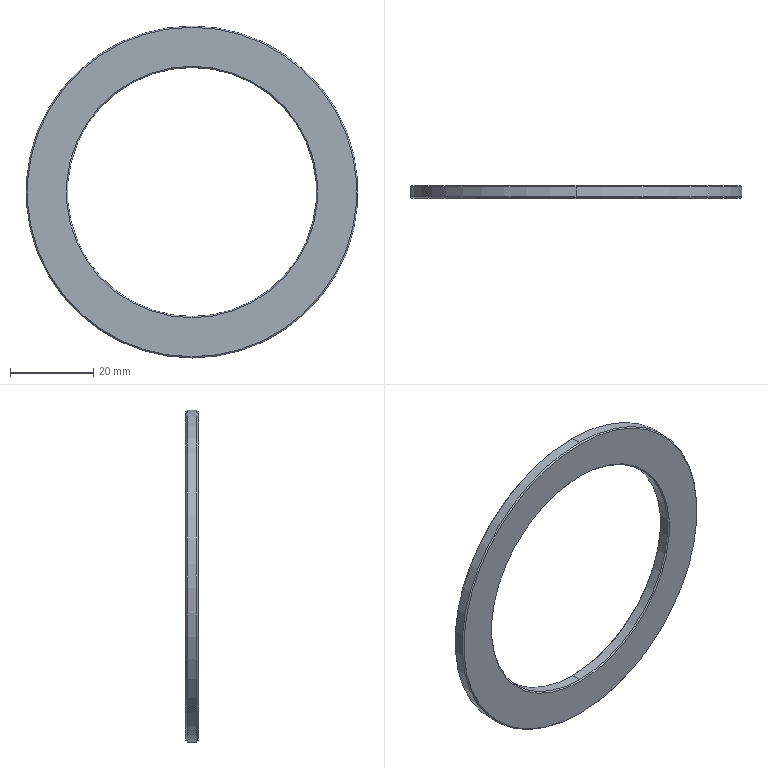Part | SolidWorks | features Chamfer 1, Extrusion 1 | 1 solid | 14 faces | box 80 x 3 x 80 mm | volume 6558 mm3 | cone 8 | cylinder 4 | plane 2 | commonest cylinder face diameters 60 x2 80 x2
STEP:
#1=CARTESIAN_POINT('',(0.,1.2,-30.));
#2=VERTEX_POINT('',#1);
#3=CARTESIAN_POINT('',(0.,1.2,30.));
#4=VERTEX_POINT('',#3);
#5=CARTESIAN_POINT('',(0.,1.2,0.));
#6=DIRECTION('',(0.,1.,0.));
#7=DIRECTION('',(0.,0.,1.));
#8=AXIS2_PLACEMENT_3D('',#5,#6,#7);
#9=CIRCLE('',#8,30.);
#10=EDGE_CURVE('',#2,#4,#9,.T.);
#11=ORIENTED_EDGE('',*,*,#10,.F.);
#12=CARTESIAN_POINT('',(0.,1.5,-30.3));
#13=VERTEX_POINT('',#12);
#14=CARTESIAN_POINT('',(0.,1.2,-30.));
#15=DIRECTION('',(0.,0.7071,-0.7071));
#16=VECTOR('',#15,1000.);
#17=LINE('',#14,#16);
#18=EDGE_CURVE('',#2,#13,#17,.T.);
#19=ORIENTED_EDGE('',*,*,#18,.T.);
#20=CARTESIAN_POINT('',(0.,1.5,30.3));
#21=VERTEX_POINT('',#20);
#22=CARTESIAN_POINT('',(0.,1.5,0.));
#23=DIRECTION('',(0.,-1.,0.));
#24=DIRECTION('',(0.,0.,1.));
#25=AXIS2_PLACEMENT_3D('',#22,#23,#24);
#26=CIRCLE('',#25,30.3);
#27=EDGE_CURVE('',#21,#13,#26,.T.);
#28=ORIENTED_EDGE('',*,*,#27,.F.);
#29=CARTESIAN_POINT('',(0.,1.2,30.));
#30=DIRECTION('',(0.,0.7071,0.7071));
#31=VECTOR('',#30,1000.);
#32=LINE('',#29,#31);
#33=EDGE_CURVE('',#4,#21,#32,.T.);
#34=ORIENTED_EDGE('',*,*,#33,.F.);
#35=EDGE_LOOP('',(#11,#19,#28,#34));
#36=FACE_OUTER_BOUND('',#35,.T.);
#37=CARTESIAN_POINT('',(0.,1.2,0.));
#38=DIRECTION('',(0.,1.,0.));
#39=DIRECTION('',(0.,0.,1.));
#40=AXIS2_PLACEMENT_3D('',#37,#38,#39);
#41=CONICAL_SURFACE('',#40,30.,0.7854);
#42=ADVANCED_FACE('',(#36),#41,.F.);
#43=CARTESIAN_POINT('',(0.,-1.2,30.));
#44=VERTEX_POINT('',#43);
#45=CARTESIAN_POINT('',(0.,-1.2,-30.));
#46=VERTEX_POINT('',#45);
#47=CARTESIAN_POINT('',(0.,-1.2,0.));
#48=DIRECTION('',(0.,-1.,0.));
#49=DIRECTION('',(0.,0.,1.));
#50=AXIS2_PLACEMENT_3D('',#47,#48,#49);
#51=CIRCLE('',#50,30.);
#52=EDGE_CURVE('',#44,#46,#51,.T.);
#53=ORIENTED_EDGE('',*,*,#52,.F.);
#54=CARTESIAN_POINT('',(0.,-1.5,30.3));
#55=VERTEX_POINT('',#54);
#56=CARTESIAN_POINT('',(0.,-1.5,30.3));
#57=DIRECTION('',(0.,-0.7071,0.7071));
#58=VECTOR('',#57,1000.);
#59=LINE('',#56,#58);
#60=EDGE_CURVE('',#44,#55,#59,.T.);
#61=ORIENTED_EDGE('',*,*,#60,.T.);
#62=CARTESIAN_POINT('',(0.,-1.5,-30.3));
#63=VERTEX_POINT('',#62);
#64=CARTESIAN_POINT('',(0.,-1.5,0.));
#65=DIRECTION('',(0.,1.,0.));
#66=DIRECTION('',(0.,0.,1.));
#67=AXIS2_PLACEMENT_3D('',#64,#65,#66);
#68=CIRCLE('',#67,30.3);
#69=EDGE_CURVE('',#63,#55,#68,.T.);
#70=ORIENTED_EDGE('',*,*,#69,.F.);
#71=CARTESIAN_POINT('',(0.,-1.5,-30.3));
#72=DIRECTION('',(0.,-0.7071,-0.7071));
#73=VECTOR('',#72,1000.);
#74=LINE('',#71,#73);
#75=EDGE_CURVE('',#46,#63,#74,.T.);
#76=ORIENTED_EDGE('',*,*,#75,.F.);
#77=EDGE_LOOP('',(#53,#61,#70,#76));
#78=FACE_OUTER_BOUND('',#77,.T.);
#79=CARTESIAN_POINT('',(0.,-1.5,0.));
#80=DIRECTION('',(0.,-1.,0.));
#81=DIRECTION('',(0.,0.,-1.));
#82=AXIS2_PLACEMENT_3D('',#79,#80,#81);
#83=CONICAL_SURFACE('',#82,30.3,0.7854);
#84=ADVANCED_FACE('',(#78),#83,.F.);
#85=CARTESIAN_POINT('',(0.,1.5,39.7));
#86=VERTEX_POINT('',#85);
#87=CARTESIAN_POINT('',(0.,1.5,-39.7));
#88=VERTEX_POINT('',#87);
#89=CARTESIAN_POINT('',(0.,1.5,0.));
#90=DIRECTION('',(0.,1.,0.));
#91=DIRECTION('',(0.,0.,1.));
#92=AXIS2_PLACEMENT_3D('',#89,#90,#91);
#93=CIRCLE('',#92,39.7);
#94=EDGE_CURVE('',#86,#88,#93,.T.);
#95=ORIENTED_EDGE('',*,*,#94,.F.);
#96=CARTESIAN_POINT('',(0.,1.2,40.));
#97=VERTEX_POINT('',#96);
#98=CARTESIAN_POINT('',(0.,1.5,39.7));
#99=DIRECTION('',(0.,-0.7071,0.7071));
#100=VECTOR('',#99,1000.);
#101=LINE('',#98,#100);
#102=EDGE_CURVE('',#86,#97,#101,.T.);
#103=ORIENTED_EDGE('',*,*,#102,.T.);
#104=CARTESIAN_POINT('',(0.,1.2,-40.));
#105=VERTEX_POINT('',#104);
#106=CARTESIAN_POINT('',(0.,1.2,0.));
#107=DIRECTION('',(0.,-1.,0.));
#108=DIRECTION('',(0.,0.,1.));
#109=AXIS2_PLACEMENT_3D('',#106,#107,#108);
#110=CIRCLE('',#109,40.);
#111=EDGE_CURVE('',#105,#97,#110,.T.);
#112=ORIENTED_EDGE('',*,*,#111,.F.);
#113=CARTESIAN_POINT('',(0.,1.5,-39.7));
#114=DIRECTION('',(0.,-0.7071,-0.7071));
#115=VECTOR('',#114,1000.);
#116=LINE('',#113,#115);
#117=EDGE_CURVE('',#88,#105,#116,.T.);
#118=ORIENTED_EDGE('',*,*,#117,.F.);
#119=EDGE_LOOP('',(#95,#103,#112,#118));
#120=FACE_OUTER_BOUND('',#119,.T.);
#121=CARTESIAN_POINT('',(0.,1.5,0.));
#122=DIRECTION('',(0.,-1.,0.));
#123=DIRECTION('',(0.,0.,-1.));
#124=AXIS2_PLACEMENT_3D('',#121,#122,#123);
#125=CONICAL_SURFACE('',#124,39.7,0.7854);
#126=ADVANCED_FACE('',(#120),#125,.T.);
#127=CARTESIAN_POINT('',(0.,-1.5,-39.7));
#128=VERTEX_POINT('',#127);
#129=CARTESIAN_POINT('',(0.,-1.5,39.7));
#130=VERTEX_POINT('',#129);
#131=CARTESIAN_POINT('',(0.,-1.5,0.));
#132=DIRECTION('',(0.,-1.,0.));
#133=DIRECTION('',(0.,0.,1.));
#134=AXIS2_PLACEMENT_3D('',#131,#132,#133);
#135=CIRCLE('',#134,39.7);
#136=EDGE_CURVE('',#128,#130,#135,.T.);
#137=ORIENTED_EDGE('',*,*,#136,.F.);
#138=CARTESIAN_POINT('',(0.,-1.2,-40.));
#139=VERTEX_POINT('',#138);
#140=CARTESIAN_POINT('',(0.,-1.2,-40.));
#141=DIRECTION('',(0.,0.7071,-0.7071));
#142=VECTOR('',#141,1000.);
#143=LINE('',#140,#142);
#144=EDGE_CURVE('',#128,#139,#143,.T.);
#145=ORIENTED_EDGE('',*,*,#144,.T.);
#146=CARTESIAN_POINT('',(0.,-1.2,40.));
#147=VERTEX_POINT('',#146);
#148=CARTESIAN_POINT('',(0.,-1.2,0.));
#149=DIRECTION('',(0.,1.,0.));
#150=DIRECTION('',(0.,0.,1.));
#151=AXIS2_PLACEMENT_3D('',#148,#149,#150);
#152=CIRCLE('',#151,40.);
#153=EDGE_CURVE('',#147,#139,#152,.T.);
#154=ORIENTED_EDGE('',*,*,#153,.F.);
#155=CARTESIAN_POINT('',(0.,-1.2,40.));
#156=DIRECTION('',(0.,0.7071,0.7071));
#157=VECTOR('',#156,1000.);
#158=LINE('',#155,#157);
#159=EDGE_CURVE('',#130,#147,#158,.T.);
#160=ORIENTED_EDGE('',*,*,#159,.F.);
#161=EDGE_LOOP('',(#137,#145,#154,#160));
#162=FACE_OUTER_BOUND('',#161,.T.);
#163=CARTESIAN_POINT('',(0.,-1.2,0.));
#164=DIRECTION('',(0.,1.,0.));
#165=DIRECTION('',(0.,0.,1.));
#166=AXIS2_PLACEMENT_3D('',#163,#164,#165);
#167=CONICAL_SURFACE('',#166,40.,0.7854);
#168=ADVANCED_FACE('',(#162),#167,.T.);
#169=ORIENTED_EDGE('',*,*,#10,.T.);
#170=CARTESIAN_POINT('',(0.,1.5,30.));
#171=DIRECTION('',(0.,-1.,0.));
#172=VECTOR('',#171,1000.);
#173=LINE('',#170,#172);
#174=EDGE_CURVE('',#4,#44,#173,.T.);
#175=ORIENTED_EDGE('',*,*,#174,.T.);
#176=ORIENTED_EDGE('',*,*,#52,.T.);
#177=CARTESIAN_POINT('',(0.,1.5,-30.));
#178=DIRECTION('',(0.,-1.,0.));
#179=VECTOR('',#178,1000.);
#180=LINE('',#177,#179);
#181=EDGE_CURVE('',#2,#46,#180,.T.);
#182=ORIENTED_EDGE('',*,*,#181,.F.);
#183=EDGE_LOOP('',(#169,#175,#176,#182));
#184=FACE_OUTER_BOUND('',#183,.T.);
#185=CARTESIAN_POINT('',(0.,1.5,0.));
#186=DIRECTION('',(0.,-1.,0.));
#187=DIRECTION('',(0.,0.,-1.));
#188=AXIS2_PLACEMENT_3D('',#185,#186,#187);
#189=CYLINDRICAL_SURFACE('',#188,30.);
#190=ADVANCED_FACE('',(#184),#189,.F.);
#191=ORIENTED_EDGE('',*,*,#111,.T.);
#192=CARTESIAN_POINT('',(0.,1.5,40.));
#193=DIRECTION('',(0.,-1.,0.));
#194=VECTOR('',#193,1000.);
#195=LINE('',#192,#194);
#196=EDGE_CURVE('',#97,#147,#195,.T.);
#197=ORIENTED_EDGE('',*,*,#196,.T.);
#198=ORIENTED_EDGE('',*,*,#153,.T.);
#199=CARTESIAN_POINT('',(0.,1.5,-40.));
#200=DIRECTION('',(0.,-1.,0.));
#201=VECTOR('',#200,1000.);
#202=LINE('',#199,#201);
#203=EDGE_CURVE('',#105,#139,#202,.T.);
#204=ORIENTED_EDGE('',*,*,#203,.F.);
#205=EDGE_LOOP('',(#191,#197,#198,#204));
#206=FACE_OUTER_BOUND('',#205,.T.);
#207=CARTESIAN_POINT('',(0.,1.5,0.));
#208=DIRECTION('',(0.,-1.,0.));
#209=DIRECTION('',(0.,0.,-1.));
#210=AXIS2_PLACEMENT_3D('',#207,#208,#209);
#211=CYLINDRICAL_SURFACE('',#210,40.);
#212=ADVANCED_FACE('',(#206),#211,.T.);
#213=CARTESIAN_POINT('',(0.,1.5,0.));
#214=DIRECTION('',(0.,1.,0.));
#215=DIRECTION('',(0.,0.,1.));
#216=AXIS2_PLACEMENT_3D('',#213,#214,#215);
#217=CIRCLE('',#216,39.7);
#218=EDGE_CURVE('',#88,#86,#217,.T.);
#219=ORIENTED_EDGE('',*,*,#218,.T.);
#220=ORIENTED_EDGE('',*,*,#94,.T.);
#221=EDGE_LOOP('',(#219,#220));
#222=FACE_OUTER_BOUND('',#221,.T.);
#223=ORIENTED_EDGE('',*,*,#27,.T.);
#224=CARTESIAN_POINT('',(0.,1.5,0.));
#225=DIRECTION('',(0.,-1.,0.));
#226=DIRECTION('',(0.,0.,1.));
#227=AXIS2_PLACEMENT_3D('',#224,#225,#226);
#228=CIRCLE('',#227,30.3);
#229=EDGE_CURVE('',#13,#21,#228,.T.);
#230=ORIENTED_EDGE('',*,*,#229,.T.);
#231=EDGE_LOOP('',(#223,#230));
#232=FACE_BOUND('',#231,.T.);
#233=CARTESIAN_POINT('',(0.,1.5,0.));
#234=DIRECTION('',(0.,1.,0.));
#235=DIRECTION('',(0.,0.,1.));
#236=AXIS2_PLACEMENT_3D('',#233,#234,#235);
#237=PLANE('',#236);
#238=ADVANCED_FACE('',(#222,#232),#237,.T.);
#239=CARTESIAN_POINT('',(0.,-1.5,0.));
#240=DIRECTION('',(0.,-1.,0.));
#241=DIRECTION('',(0.,0.,1.));
#242=AXIS2_PLACEMENT_3D('',#239,#240,#241);
#243=CIRCLE('',#242,39.7);
#244=EDGE_CURVE('',#130,#128,#243,.T.);
#245=ORIENTED_EDGE('',*,*,#244,.T.);
#246=ORIENTED_EDGE('',*,*,#136,.T.);
#247=EDGE_LOOP('',(#245,#246));
#248=FACE_OUTER_BOUND('',#247,.T.);
#249=ORIENTED_EDGE('',*,*,#69,.T.);
#250=CARTESIAN_POINT('',(0.,-1.5,0.));
#251=DIRECTION('',(0.,1.,0.));
#252=DIRECTION('',(0.,0.,1.));
#253=AXIS2_PLACEMENT_3D('',#250,#251,#252);
#254=CIRCLE('',#253,30.3);
#255=EDGE_CURVE('',#55,#63,#254,.T.);
#256=ORIENTED_EDGE('',*,*,#255,.T.);
#257=EDGE_LOOP('',(#249,#256));
#258=FACE_BOUND('',#257,.T.);
#259=CARTESIAN_POINT('',(0.,-1.5,0.));
#260=DIRECTION('',(0.,1.,0.));
#261=DIRECTION('',(0.,0.,1.));
#262=AXIS2_PLACEMENT_3D('',#259,#260,#261);
#263=PLANE('',#262);
#264=ADVANCED_FACE('',(#248,#258),#263,.F.);
#265=ORIENTED_EDGE('',*,*,#196,.F.);
#266=CARTESIAN_POINT('',(0.,1.2,0.));
#267=DIRECTION('',(0.,-1.,0.));
#268=DIRECTION('',(0.,0.,1.));
#269=AXIS2_PLACEMENT_3D('',#266,#267,#268);
#270=CIRCLE('',#269,40.);
#271=EDGE_CURVE('',#97,#105,#270,.T.);
#272=ORIENTED_EDGE('',*,*,#271,.T.);
#273=ORIENTED_EDGE('',*,*,#203,.T.);
#274=CARTESIAN_POINT('',(0.,-1.2,0.));
#275=DIRECTION('',(0.,1.,0.));
#276=DIRECTION('',(0.,0.,1.));
#277=AXIS2_PLACEMENT_3D('',#274,#275,#276);
#278=CIRCLE('',#277,40.);
#279=EDGE_CURVE('',#139,#147,#278,.T.);
#280=ORIENTED_EDGE('',*,*,#279,.T.);
#281=EDGE_LOOP('',(#265,#272,#273,#280));
#282=FACE_OUTER_BOUND('',#281,.T.);
#283=CARTESIAN_POINT('',(0.,1.5,0.));
#284=DIRECTION('',(0.,-1.,0.));
#285=DIRECTION('',(0.,0.,-1.));
#286=AXIS2_PLACEMENT_3D('',#283,#284,#285);
#287=CYLINDRICAL_SURFACE('',#286,40.);
#288=ADVANCED_FACE('',(#282),#287,.T.);
#289=ORIENTED_EDGE('',*,*,#174,.F.);
#290=CARTESIAN_POINT('',(0.,1.2,0.));
#291=DIRECTION('',(0.,1.,0.));
#292=DIRECTION('',(0.,0.,1.));
#293=AXIS2_PLACEMENT_3D('',#290,#291,#292);
#294=CIRCLE('',#293,30.);
#295=EDGE_CURVE('',#4,#2,#294,.T.);
#296=ORIENTED_EDGE('',*,*,#295,.T.);
#297=ORIENTED_EDGE('',*,*,#181,.T.);
#298=CARTESIAN_POINT('',(0.,-1.2,0.));
#299=DIRECTION('',(0.,-1.,0.));
#300=DIRECTION('',(0.,0.,1.));
#301=AXIS2_PLACEMENT_3D('',#298,#299,#300);
#302=CIRCLE('',#301,30.);
#303=EDGE_CURVE('',#46,#44,#302,.T.);
#304=ORIENTED_EDGE('',*,*,#303,.T.);
#305=EDGE_LOOP('',(#289,#296,#297,#304));
#306=FACE_OUTER_BOUND('',#305,.T.);
#307=CARTESIAN_POINT('',(0.,1.5,0.));
#308=DIRECTION('',(0.,-1.,0.));
#309=DIRECTION('',(0.,0.,-1.));
#310=AXIS2_PLACEMENT_3D('',#307,#308,#309);
#311=CYLINDRICAL_SURFACE('',#310,30.);
#312=ADVANCED_FACE('',(#306),#311,.F.);
#313=ORIENTED_EDGE('',*,*,#144,.F.);
#314=ORIENTED_EDGE('',*,*,#244,.F.);
#315=ORIENTED_EDGE('',*,*,#159,.T.);
#316=ORIENTED_EDGE('',*,*,#279,.F.);
#317=EDGE_LOOP('',(#313,#314,#315,#316));
#318=FACE_OUTER_BOUND('',#317,.T.);
#319=CARTESIAN_POINT('',(0.,-1.2,0.));
#320=DIRECTION('',(0.,1.,0.));
#321=DIRECTION('',(0.,0.,1.));
#322=AXIS2_PLACEMENT_3D('',#319,#320,#321);
#323=CONICAL_SURFACE('',#322,40.,0.7854);
#324=ADVANCED_FACE('',(#318),#323,.T.);
#325=ORIENTED_EDGE('',*,*,#102,.F.);
#326=ORIENTED_EDGE('',*,*,#218,.F.);
#327=ORIENTED_EDGE('',*,*,#117,.T.);
#328=ORIENTED_EDGE('',*,*,#271,.F.);
#329=EDGE_LOOP('',(#325,#326,#327,#328));
#330=FACE_OUTER_BOUND('',#329,.T.);
#331=CARTESIAN_POINT('',(0.,1.5,0.));
#332=DIRECTION('',(0.,-1.,0.));
#333=DIRECTION('',(0.,0.,-1.));
#334=AXIS2_PLACEMENT_3D('',#331,#332,#333);
#335=CONICAL_SURFACE('',#334,39.7,0.7854);
#336=ADVANCED_FACE('',(#330),#335,.T.);
#337=ORIENTED_EDGE('',*,*,#60,.F.);
#338=ORIENTED_EDGE('',*,*,#303,.F.);
#339=ORIENTED_EDGE('',*,*,#75,.T.);
#340=ORIENTED_EDGE('',*,*,#255,.F.);
#341=EDGE_LOOP('',(#337,#338,#339,#340));
#342=FACE_OUTER_BOUND('',#341,.T.);
#343=CARTESIAN_POINT('',(0.,-1.5,0.));
#344=DIRECTION('',(0.,-1.,0.));
#345=DIRECTION('',(0.,0.,-1.));
#346=AXIS2_PLACEMENT_3D('',#343,#344,#345);
#347=CONICAL_SURFACE('',#346,30.3,0.7854);
#348=ADVANCED_FACE('',(#342),#347,.F.);
#349=ORIENTED_EDGE('',*,*,#18,.F.);
#350=ORIENTED_EDGE('',*,*,#295,.F.);
#351=ORIENTED_EDGE('',*,*,#33,.T.);
#352=ORIENTED_EDGE('',*,*,#229,.F.);
#353=EDGE_LOOP('',(#349,#350,#351,#352));
#354=FACE_OUTER_BOUND('',#353,.T.);
#355=CARTESIAN_POINT('',(0.,1.2,0.));
#356=DIRECTION('',(0.,1.,0.));
#357=DIRECTION('',(0.,0.,1.));
#358=AXIS2_PLACEMENT_3D('',#355,#356,#357);
#359=CONICAL_SURFACE('',#358,30.,0.7854);
#360=ADVANCED_FACE('',(#354),#359,.F.);
#361=CLOSED_SHELL('',(#42,#84,#126,#168,#190,#212,#238,#264,#288,#312,#324,#336,#348,#360));
#362=MANIFOLD_SOLID_BREP('',#361);
#363=CARTESIAN_POINT('',(0.,0.,0.));
#364=DIRECTION('',(0.,0.,1.));
#365=DIRECTION('',(1.,0.,0.));
#366=AXIS2_PLACEMENT_3D('',#363,#364,#365);
#367=(LENGTH_UNIT()NAMED_UNIT(*)SI_UNIT(.MILLI.,.METRE.));
#368=UNCERTAINTY_MEASURE_WITH_UNIT(LENGTH_MEASURE(0.00001),#367,'','');
#369=(NAMED_UNIT(*)PLANE_ANGLE_UNIT()SI_UNIT($,.RADIAN.));
#370=(NAMED_UNIT(*)SI_UNIT($,.STERADIAN.)SOLID_ANGLE_UNIT());
#371=(GEOMETRIC_REPRESENTATION_CONTEXT(3)GLOBAL_UNCERTAINTY_ASSIGNED_CONTEXT((#368))GLOBAL_UNIT_ASSIGNED_CONTEXT((#367,#369,#370))REPRESENTATION_CONTEXT('',''));
#372=ADVANCED_BREP_SHAPE_REPRESENTATION('',(#362,#366),#371);